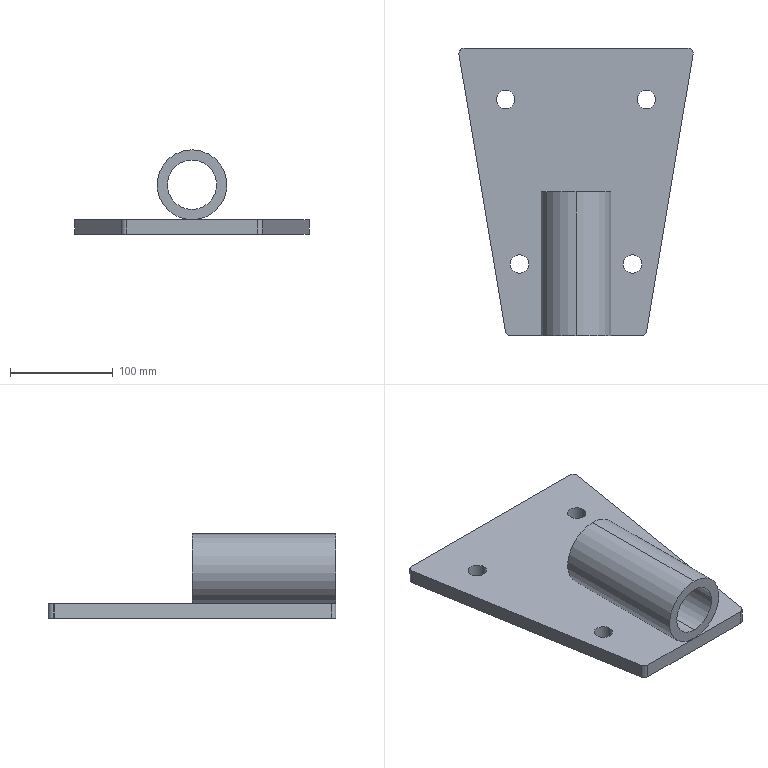Part | SolidWorks | features Extrusion 1, Fillet 1, HoleWzd 1, ICE 1 | 2 solids | 25 faces | box 227.837 x 280 x 82 mm | volume 957079 mm3 | cylinder 17 | plane 8 | commonest cylinder face diameters 18 x8 10 x5 48 x2 68 x2
STEP:
#1=CARTESIAN_POINT('',(0.,-2195.,72.));
#2=VERTEX_POINT('',#1);
#3=CARTESIAN_POINT('',(0.,-2195.,24.));
#4=VERTEX_POINT('',#3);
#5=CARTESIAN_POINT('',(0.,-2195.,48.));
#6=DIRECTION('',(0.,-1.,0.));
#7=DIRECTION('',(0.,0.,-1.));
#8=AXIS2_PLACEMENT_3D('',#5,#6,#7);
#9=CIRCLE('',#8,24.);
#10=EDGE_CURVE('',#2,#4,#9,.T.);
#11=ORIENTED_EDGE('',*,*,#10,.F.);
#12=CARTESIAN_POINT('',(0.,-2335.,72.));
#13=VERTEX_POINT('',#12);
#14=CARTESIAN_POINT('',(0.,-2195.,72.));
#15=DIRECTION('',(0.,-1.,0.));
#16=VECTOR('',#15,1000.);
#17=LINE('',#14,#16);
#18=EDGE_CURVE('',#2,#13,#17,.T.);
#19=ORIENTED_EDGE('',*,*,#18,.T.);
#20=CARTESIAN_POINT('',(0.,-2335.,24.));
#21=VERTEX_POINT('',#20);
#22=CARTESIAN_POINT('',(0.,-2335.,48.));
#23=DIRECTION('',(0.,-1.,0.));
#24=DIRECTION('',(0.,0.,-1.));
#25=AXIS2_PLACEMENT_3D('',#22,#23,#24);
#26=CIRCLE('',#25,24.);
#27=EDGE_CURVE('',#13,#21,#26,.T.);
#28=ORIENTED_EDGE('',*,*,#27,.T.);
#29=CARTESIAN_POINT('',(0.,-2195.,24.));
#30=DIRECTION('',(0.,-1.,0.));
#31=VECTOR('',#30,1000.);
#32=LINE('',#29,#31);
#33=EDGE_CURVE('',#4,#21,#32,.T.);
#34=ORIENTED_EDGE('',*,*,#33,.F.);
#35=EDGE_LOOP('',(#11,#19,#28,#34));
#36=FACE_OUTER_BOUND('',#35,.T.);
#37=CARTESIAN_POINT('',(0.,-2195.,48.));
#38=DIRECTION('',(0.,-1.,0.));
#39=DIRECTION('',(0.,0.,-1.));
#40=AXIS2_PLACEMENT_3D('',#37,#38,#39);
#41=CYLINDRICAL_SURFACE('',#40,24.);
#42=ADVANCED_FACE('',(#36),#41,.F.);
#43=CARTESIAN_POINT('',(0.,-2195.,14.));
#44=VERTEX_POINT('',#43);
#45=CARTESIAN_POINT('',(0.,-2195.,82.));
#46=VERTEX_POINT('',#45);
#47=CARTESIAN_POINT('',(0.,-2195.,48.));
#48=DIRECTION('',(0.,-1.,0.));
#49=DIRECTION('',(0.,0.,-1.));
#50=AXIS2_PLACEMENT_3D('',#47,#48,#49);
#51=CIRCLE('',#50,34.);
#52=EDGE_CURVE('',#44,#46,#51,.T.);
#53=ORIENTED_EDGE('',*,*,#52,.T.);
#54=CARTESIAN_POINT('',(0.,-2335.,82.));
#55=VERTEX_POINT('',#54);
#56=CARTESIAN_POINT('',(0.,-2195.,82.));
#57=DIRECTION('',(0.,-1.,0.));
#58=VECTOR('',#57,1000.);
#59=LINE('',#56,#58);
#60=EDGE_CURVE('',#46,#55,#59,.T.);
#61=ORIENTED_EDGE('',*,*,#60,.T.);
#62=CARTESIAN_POINT('',(0.,-2335.,14.));
#63=VERTEX_POINT('',#62);
#64=CARTESIAN_POINT('',(0.,-2335.,48.));
#65=DIRECTION('',(0.,-1.,0.));
#66=DIRECTION('',(0.,0.,-1.));
#67=AXIS2_PLACEMENT_3D('',#64,#65,#66);
#68=CIRCLE('',#67,34.);
#69=EDGE_CURVE('',#63,#55,#68,.T.);
#70=ORIENTED_EDGE('',*,*,#69,.F.);
#71=CARTESIAN_POINT('',(0.,-2195.,14.));
#72=DIRECTION('',(0.,-1.,0.));
#73=VECTOR('',#72,1000.);
#74=LINE('',#71,#73);
#75=EDGE_CURVE('',#44,#63,#74,.T.);
#76=ORIENTED_EDGE('',*,*,#75,.F.);
#77=EDGE_LOOP('',(#53,#61,#70,#76));
#78=FACE_OUTER_BOUND('',#77,.T.);
#79=CARTESIAN_POINT('',(0.,-2195.,48.));
#80=DIRECTION('',(0.,-1.,0.));
#81=DIRECTION('',(0.,0.,-1.));
#82=AXIS2_PLACEMENT_3D('',#79,#80,#81);
#83=CYLINDRICAL_SURFACE('',#82,34.);
#84=ADVANCED_FACE('',(#78),#83,.T.);
#85=ORIENTED_EDGE('',*,*,#60,.F.);
#86=CARTESIAN_POINT('',(0.,-2195.,48.));
#87=DIRECTION('',(0.,-1.,0.));
#88=DIRECTION('',(0.,0.,-1.));
#89=AXIS2_PLACEMENT_3D('',#86,#87,#88);
#90=CIRCLE('',#89,34.);
#91=EDGE_CURVE('',#46,#44,#90,.T.);
#92=ORIENTED_EDGE('',*,*,#91,.T.);
#93=ORIENTED_EDGE('',*,*,#75,.T.);
#94=CARTESIAN_POINT('',(0.,-2335.,48.));
#95=DIRECTION('',(0.,-1.,0.));
#96=DIRECTION('',(0.,0.,-1.));
#97=AXIS2_PLACEMENT_3D('',#94,#95,#96);
#98=CIRCLE('',#97,34.);
#99=EDGE_CURVE('',#55,#63,#98,.T.);
#100=ORIENTED_EDGE('',*,*,#99,.F.);
#101=EDGE_LOOP('',(#85,#92,#93,#100));
#102=FACE_OUTER_BOUND('',#101,.T.);
#103=CARTESIAN_POINT('',(0.,-2195.,48.));
#104=DIRECTION('',(0.,-1.,0.));
#105=DIRECTION('',(0.,0.,-1.));
#106=AXIS2_PLACEMENT_3D('',#103,#104,#105);
#107=CYLINDRICAL_SURFACE('',#106,34.);
#108=ADVANCED_FACE('',(#102),#107,.T.);
#109=CARTESIAN_POINT('',(0.,-2195.,48.));
#110=DIRECTION('',(0.,-1.,0.));
#111=DIRECTION('',(0.,0.,-1.));
#112=AXIS2_PLACEMENT_3D('',#109,#110,#111);
#113=CIRCLE('',#112,24.);
#114=EDGE_CURVE('',#4,#2,#113,.T.);
#115=ORIENTED_EDGE('',*,*,#114,.T.);
#116=ORIENTED_EDGE('',*,*,#10,.T.);
#117=EDGE_LOOP('',(#115,#116));
#118=FACE_BOUND('',#117,.T.);
#119=ORIENTED_EDGE('',*,*,#52,.F.);
#120=ORIENTED_EDGE('',*,*,#91,.F.);
#121=EDGE_LOOP('',(#119,#120));
#122=FACE_OUTER_BOUND('',#121,.T.);
#123=CARTESIAN_POINT('',(0.,-2195.,48.));
#124=DIRECTION('',(0.,-1.,0.));
#125=DIRECTION('',(0.,0.,-1.));
#126=AXIS2_PLACEMENT_3D('',#123,#124,#125);
#127=PLANE('',#126);
#128=ADVANCED_FACE('',(#118,#122),#127,.F.);
#129=CARTESIAN_POINT('',(0.,-2335.,48.));
#130=DIRECTION('',(0.,-1.,0.));
#131=DIRECTION('',(0.,0.,-1.));
#132=AXIS2_PLACEMENT_3D('',#129,#130,#131);
#133=CIRCLE('',#132,24.);
#134=EDGE_CURVE('',#21,#13,#133,.T.);
#135=ORIENTED_EDGE('',*,*,#134,.F.);
#136=ORIENTED_EDGE('',*,*,#27,.F.);
#137=EDGE_LOOP('',(#135,#136));
#138=FACE_BOUND('',#137,.T.);
#139=ORIENTED_EDGE('',*,*,#69,.T.);
#140=ORIENTED_EDGE('',*,*,#99,.T.);
#141=EDGE_LOOP('',(#139,#140));
#142=FACE_OUTER_BOUND('',#141,.T.);
#143=CARTESIAN_POINT('',(0.,-2335.,48.));
#144=DIRECTION('',(0.,-1.,0.));
#145=DIRECTION('',(0.,0.,-1.));
#146=AXIS2_PLACEMENT_3D('',#143,#144,#145);
#147=PLANE('',#146);
#148=ADVANCED_FACE('',(#138,#142),#147,.T.);
#149=ORIENTED_EDGE('',*,*,#18,.F.);
#150=ORIENTED_EDGE('',*,*,#114,.F.);
#151=ORIENTED_EDGE('',*,*,#33,.T.);
#152=ORIENTED_EDGE('',*,*,#134,.T.);
#153=EDGE_LOOP('',(#149,#150,#151,#152));
#154=FACE_OUTER_BOUND('',#153,.T.);
#155=CARTESIAN_POINT('',(0.,-2195.,48.));
#156=DIRECTION('',(0.,-1.,0.));
#157=DIRECTION('',(0.,0.,-1.));
#158=AXIS2_PLACEMENT_3D('',#155,#156,#157);
#159=CYLINDRICAL_SURFACE('',#158,24.);
#160=ADVANCED_FACE('',(#154),#159,.F.);
#161=CLOSED_SHELL('',(#42,#84,#108,#128,#148,#160));
#162=MANIFOLD_SOLID_BREP('',#161);
#163=CARTESIAN_POINT('',(59.437,-2105.,14.));
#164=VERTEX_POINT('',#163);
#165=CARTESIAN_POINT('',(77.437,-2105.,14.));
#166=VERTEX_POINT('',#165);
#167=CARTESIAN_POINT('',(68.437,-2105.,14.));
#168=DIRECTION('',(0.,0.,1.));
#169=DIRECTION('',(1.,0.,0.));
#170=AXIS2_PLACEMENT_3D('',#167,#168,#169);
#171=CIRCLE('',#170,9.);
#172=EDGE_CURVE('',#164,#166,#171,.T.);
#173=ORIENTED_EDGE('',*,*,#172,.T.);
#174=CARTESIAN_POINT('',(77.437,-2105.,0.));
#175=VERTEX_POINT('',#174);
#176=CARTESIAN_POINT('',(77.437,-2105.,0.));
#177=DIRECTION('',(0.,0.,-1.));
#178=VECTOR('',#177,1000.);
#179=LINE('',#176,#178);
#180=EDGE_CURVE('',#166,#175,#179,.T.);
#181=ORIENTED_EDGE('',*,*,#180,.T.);
#182=CARTESIAN_POINT('',(59.437,-2105.,0.));
#183=VERTEX_POINT('',#182);
#184=CARTESIAN_POINT('',(68.437,-2105.,0.));
#185=DIRECTION('',(0.,0.,-1.));
#186=DIRECTION('',(-1.,0.,0.));
#187=AXIS2_PLACEMENT_3D('',#184,#185,#186);
#188=CIRCLE('',#187,9.);
#189=EDGE_CURVE('',#175,#183,#188,.T.);
#190=ORIENTED_EDGE('',*,*,#189,.T.);
#191=CARTESIAN_POINT('',(59.437,-2105.,0.));
#192=DIRECTION('',(0.,0.,-1.));
#193=VECTOR('',#192,1000.);
#194=LINE('',#191,#193);
#195=EDGE_CURVE('',#164,#183,#194,.T.);
#196=ORIENTED_EDGE('',*,*,#195,.F.);
#197=EDGE_LOOP('',(#173,#181,#190,#196));
#198=FACE_OUTER_BOUND('',#197,.T.);
#199=CARTESIAN_POINT('',(68.437,-2105.,0.));
#200=DIRECTION('',(0.,0.,-1.));
#201=DIRECTION('',(-1.,0.,0.));
#202=AXIS2_PLACEMENT_3D('',#199,#200,#201);
#203=CYLINDRICAL_SURFACE('',#202,9.);
#204=ADVANCED_FACE('',(#198),#203,.F.);
#205=CARTESIAN_POINT('',(46.,-2265.,14.));
#206=VERTEX_POINT('',#205);
#207=CARTESIAN_POINT('',(64.,-2265.,14.));
#208=VERTEX_POINT('',#207);
#209=CARTESIAN_POINT('',(55.,-2265.,14.));
#210=DIRECTION('',(0.,0.,1.));
#211=DIRECTION('',(1.,0.,0.));
#212=AXIS2_PLACEMENT_3D('',#209,#210,#211);
#213=CIRCLE('',#212,9.);
#214=EDGE_CURVE('',#206,#208,#213,.T.);
#215=ORIENTED_EDGE('',*,*,#214,.T.);
#216=CARTESIAN_POINT('',(64.,-2265.,0.));
#217=VERTEX_POINT('',#216);
#218=CARTESIAN_POINT('',(64.,-2265.,0.));
#219=DIRECTION('',(0.,0.,-1.));
#220=VECTOR('',#219,1000.);
#221=LINE('',#218,#220);
#222=EDGE_CURVE('',#208,#217,#221,.T.);
#223=ORIENTED_EDGE('',*,*,#222,.T.);
#224=CARTESIAN_POINT('',(46.,-2265.,0.));
#225=VERTEX_POINT('',#224);
#226=CARTESIAN_POINT('',(55.,-2265.,0.));
#227=DIRECTION('',(0.,0.,-1.));
#228=DIRECTION('',(-1.,0.,0.));
#229=AXIS2_PLACEMENT_3D('',#226,#227,#228);
#230=CIRCLE('',#229,9.);
#231=EDGE_CURVE('',#217,#225,#230,.T.);
#232=ORIENTED_EDGE('',*,*,#231,.T.);
#233=CARTESIAN_POINT('',(46.,-2265.,0.));
#234=DIRECTION('',(0.,0.,-1.));
#235=VECTOR('',#234,1000.);
#236=LINE('',#233,#235);
#237=EDGE_CURVE('',#206,#225,#236,.T.);
#238=ORIENTED_EDGE('',*,*,#237,.F.);
#239=EDGE_LOOP('',(#215,#223,#232,#238));
#240=FACE_OUTER_BOUND('',#239,.T.);
#241=CARTESIAN_POINT('',(55.,-2265.,0.));
#242=DIRECTION('',(0.,0.,-1.));
#243=DIRECTION('',(-1.,0.,0.));
#244=AXIS2_PLACEMENT_3D('',#241,#242,#243);
#245=CYLINDRICAL_SURFACE('',#244,9.);
#246=ADVANCED_FACE('',(#240),#245,.F.);
#247=CARTESIAN_POINT('',(-64.,-2265.,14.));
#248=VERTEX_POINT('',#247);
#249=CARTESIAN_POINT('',(-46.,-2265.,14.));
#250=VERTEX_POINT('',#249);
#251=CARTESIAN_POINT('',(-55.,-2265.,14.));
#252=DIRECTION('',(0.,0.,1.));
#253=DIRECTION('',(1.,0.,0.));
#254=AXIS2_PLACEMENT_3D('',#251,#252,#253);
#255=CIRCLE('',#254,9.);
#256=EDGE_CURVE('',#248,#250,#255,.T.);
#257=ORIENTED_EDGE('',*,*,#256,.T.);
#258=CARTESIAN_POINT('',(-46.,-2265.,0.));
#259=VERTEX_POINT('',#258);
#260=CARTESIAN_POINT('',(-46.,-2265.,0.));
#261=DIRECTION('',(0.,0.,-1.));
#262=VECTOR('',#261,1000.);
#263=LINE('',#260,#262);
#264=EDGE_CURVE('',#250,#259,#263,.T.);
#265=ORIENTED_EDGE('',*,*,#264,.T.);
#266=CARTESIAN_POINT('',(-64.,-2265.,0.));
#267=VERTEX_POINT('',#266);
#268=CARTESIAN_POINT('',(-55.,-2265.,0.));
#269=DIRECTION('',(0.,0.,-1.));
#270=DIRECTION('',(-1.,0.,0.));
#271=AXIS2_PLACEMENT_3D('',#268,#269,#270);
#272=CIRCLE('',#271,9.);
#273=EDGE_CURVE('',#259,#267,#272,.T.);
#274=ORIENTED_EDGE('',*,*,#273,.T.);
#275=CARTESIAN_POINT('',(-64.,-2265.,0.));
#276=DIRECTION('',(0.,0.,-1.));
#277=VECTOR('',#276,1000.);
#278=LINE('',#275,#277);
#279=EDGE_CURVE('',#248,#267,#278,.T.);
#280=ORIENTED_EDGE('',*,*,#279,.F.);
#281=EDGE_LOOP('',(#257,#265,#274,#280));
#282=FACE_OUTER_BOUND('',#281,.T.);
#283=CARTESIAN_POINT('',(-55.,-2265.,0.));
#284=DIRECTION('',(0.,0.,-1.));
#285=DIRECTION('',(-1.,0.,0.));
#286=AXIS2_PLACEMENT_3D('',#283,#284,#285);
#287=CYLINDRICAL_SURFACE('',#286,9.);
#288=ADVANCED_FACE('',(#282),#287,.F.);
#289=CARTESIAN_POINT('',(-77.437,-2105.,14.));
#290=VERTEX_POINT('',#289);
#291=CARTESIAN_POINT('',(-59.437,-2105.,14.));
#292=VERTEX_POINT('',#291);
#293=CARTESIAN_POINT('',(-68.437,-2105.,14.));
#294=DIRECTION('',(0.,0.,1.));
#295=DIRECTION('',(1.,0.,0.));
#296=AXIS2_PLACEMENT_3D('',#293,#294,#295);
#297=CIRCLE('',#296,9.);
#298=EDGE_CURVE('',#290,#292,#297,.T.);
#299=ORIENTED_EDGE('',*,*,#298,.T.);
#300=CARTESIAN_POINT('',(-59.437,-2105.,0.));
#301=VERTEX_POINT('',#300);
#302=CARTESIAN_POINT('',(-59.437,-2105.,0.));
#303=DIRECTION('',(0.,0.,-1.));
#304=VECTOR('',#303,1000.);
#305=LINE('',#302,#304);
#306=EDGE_CURVE('',#292,#301,#305,.T.);
#307=ORIENTED_EDGE('',*,*,#306,.T.);
#308=CARTESIAN_POINT('',(-77.437,-2105.,0.));
#309=VERTEX_POINT('',#308);
#310=CARTESIAN_POINT('',(-68.437,-2105.,0.));
#311=DIRECTION('',(0.,0.,-1.));
#312=DIRECTION('',(-1.,0.,0.));
#313=AXIS2_PLACEMENT_3D('',#310,#311,#312);
#314=CIRCLE('',#313,9.);
#315=EDGE_CURVE('',#301,#309,#314,.T.);
#316=ORIENTED_EDGE('',*,*,#315,.T.);
#317=CARTESIAN_POINT('',(-77.437,-2105.,0.));
#318=DIRECTION('',(0.,0.,-1.));
#319=VECTOR('',#318,1000.);
#320=LINE('',#317,#319);
#321=EDGE_CURVE('',#290,#309,#320,.T.);
#322=ORIENTED_EDGE('',*,*,#321,.F.);
#323=EDGE_LOOP('',(#299,#307,#316,#322));
#324=FACE_OUTER_BOUND('',#323,.T.);
#325=CARTESIAN_POINT('',(-68.437,-2105.,0.));
#326=DIRECTION('',(0.,0.,-1.));
#327=DIRECTION('',(-1.,0.,0.));
#328=AXIS2_PLACEMENT_3D('',#325,#326,#327);
#329=CYLINDRICAL_SURFACE('',#328,9.);
#330=ADVANCED_FACE('',(#324),#329,.F.);
#331=CARTESIAN_POINT('',(-113.919,-2060.,14.));
#332=VERTEX_POINT('',#331);
#333=CARTESIAN_POINT('',(-113.85,-2060.825,14.));
#334=VERTEX_POINT('',#333);
#335=CARTESIAN_POINT('',(-108.919,-2060.,14.));
#336=DIRECTION('',(0.,0.,1.));
#337=DIRECTION('',(1.,0.,0.));
#338=AXIS2_PLACEMENT_3D('',#335,#336,#337);
#339=CIRCLE('',#338,5.);
#340=EDGE_CURVE('',#332,#334,#339,.T.);
#341=ORIENTED_EDGE('',*,*,#340,.F.);
#342=CARTESIAN_POINT('',(-113.919,-2060.,0.));
#343=VERTEX_POINT('',#342);
#344=CARTESIAN_POINT('',(-113.919,-2060.,14.));
#345=DIRECTION('',(0.,0.,-1.));
#346=VECTOR('',#345,1000.);
#347=LINE('',#344,#346);
#348=EDGE_CURVE('',#332,#343,#347,.T.);
#349=ORIENTED_EDGE('',*,*,#348,.T.);
#350=CARTESIAN_POINT('',(-113.85,-2060.825,0.));
#351=VERTEX_POINT('',#350);
#352=CARTESIAN_POINT('',(-108.919,-2060.,0.));
#353=DIRECTION('',(0.,0.,-1.));
#354=DIRECTION('',(1.,0.,0.));
#355=AXIS2_PLACEMENT_3D('',#352,#353,#354);
#356=CIRCLE('',#355,5.);
#357=EDGE_CURVE('',#351,#343,#356,.T.);
#358=ORIENTED_EDGE('',*,*,#357,.F.);
#359=CARTESIAN_POINT('',(-113.85,-2060.825,14.));
#360=DIRECTION('',(0.,0.,-1.));
#361=VECTOR('',#360,1000.);
#362=LINE('',#359,#361);
#363=EDGE_CURVE('',#334,#351,#362,.T.);
#364=ORIENTED_EDGE('',*,*,#363,.F.);
#365=EDGE_LOOP('',(#341,#349,#358,#364));
#366=FACE_OUTER_BOUND('',#365,.T.);
#367=CARTESIAN_POINT('',(-108.919,-2060.,14.));
#368=DIRECTION('',(0.,0.,-1.));
#369=DIRECTION('',(-1.,0.,0.));
#370=AXIS2_PLACEMENT_3D('',#367,#368,#369);
#371=CYLINDRICAL_SURFACE('',#370,5.);
#372=ADVANCED_FACE('',(#366),#371,.T.);
#373=CARTESIAN_POINT('',(-68.668,-2330.825,14.));
#374=VERTEX_POINT('',#373);
#375=CARTESIAN_POINT('',(-114.825,-2055.,14.));
#376=DIRECTION('',(0.165,-0.9863,0.));
#377=VECTOR('',#376,1000.);
#378=LINE('',#375,#377);
#379=EDGE_CURVE('',#334,#374,#378,.T.);
#380=ORIENTED_EDGE('',*,*,#379,.F.);
#381=ORIENTED_EDGE('',*,*,#363,.T.);
#382=CARTESIAN_POINT('',(-68.668,-2330.825,0.));
#383=VERTEX_POINT('',#382);
#384=CARTESIAN_POINT('',(-114.825,-2055.,0.));
#385=DIRECTION('',(0.165,-0.9863,0.));
#386=VECTOR('',#385,1000.);
#387=LINE('',#384,#386);
#388=EDGE_CURVE('',#351,#383,#387,.T.);
#389=ORIENTED_EDGE('',*,*,#388,.T.);
#390=CARTESIAN_POINT('',(-68.668,-2330.825,14.));
#391=DIRECTION('',(0.,0.,1.));
#392=VECTOR('',#391,1000.);
#393=LINE('',#390,#392);
#394=EDGE_CURVE('',#383,#374,#393,.T.);
#395=ORIENTED_EDGE('',*,*,#394,.T.);
#396=EDGE_LOOP('',(#380,#381,#389,#395));
#397=FACE_OUTER_BOUND('',#396,.T.);
#398=CARTESIAN_POINT('',(-114.825,-2055.,14.));
#399=DIRECTION('',(0.9863,0.165,0.));
#400=DIRECTION('',(-0.165,0.9863,0.));
#401=AXIS2_PLACEMENT_3D('',#398,#399,#400);
#402=PLANE('',#401);
#403=ADVANCED_FACE('',(#397),#402,.F.);
#404=CARTESIAN_POINT('',(-63.736,-2335.,14.));
#405=VERTEX_POINT('',#404);
#406=CARTESIAN_POINT('',(63.736,-2335.,14.));
#407=VERTEX_POINT('',#406);
#408=CARTESIAN_POINT('',(-67.969,-2335.,14.));
#409=DIRECTION('',(1.,0.,0.));
#410=VECTOR('',#409,1000.);
#411=LINE('',#408,#410);
#412=EDGE_CURVE('',#405,#407,#411,.T.);
#413=ORIENTED_EDGE('',*,*,#412,.F.);
#414=CARTESIAN_POINT('',(-63.736,-2335.,0.));
#415=VERTEX_POINT('',#414);
#416=CARTESIAN_POINT('',(-63.736,-2335.,14.));
#417=DIRECTION('',(0.,0.,-1.));
#418=VECTOR('',#417,1000.);
#419=LINE('',#416,#418);
#420=EDGE_CURVE('',#405,#415,#419,.T.);
#421=ORIENTED_EDGE('',*,*,#420,.T.);
#422=CARTESIAN_POINT('',(63.736,-2335.,0.));
#423=VERTEX_POINT('',#422);
#424=CARTESIAN_POINT('',(-67.969,-2335.,0.));
#425=DIRECTION('',(1.,0.,0.));
#426=VECTOR('',#425,1000.);
#427=LINE('',#424,#426);
#428=EDGE_CURVE('',#415,#423,#427,.T.);
#429=ORIENTED_EDGE('',*,*,#428,.T.);
#430=CARTESIAN_POINT('',(63.736,-2335.,14.));
#431=DIRECTION('',(0.,0.,1.));
#432=VECTOR('',#431,1000.);
#433=LINE('',#430,#432);
#434=EDGE_CURVE('',#423,#407,#433,.T.);
#435=ORIENTED_EDGE('',*,*,#434,.T.);
#436=EDGE_LOOP('',(#413,#421,#429,#435));
#437=FACE_OUTER_BOUND('',#436,.T.);
#438=CARTESIAN_POINT('',(-67.969,-2335.,14.));
#439=DIRECTION('',(0.,1.,0.));
#440=DIRECTION('',(0.,0.,1.));
#441=AXIS2_PLACEMENT_3D('',#438,#439,#440);
#442=PLANE('',#441);
#443=ADVANCED_FACE('',(#437),#442,.F.);
#444=CARTESIAN_POINT('',(68.668,-2330.825,0.));
#445=VERTEX_POINT('',#444);
#446=CARTESIAN_POINT('',(113.85,-2060.825,0.));
#447=VERTEX_POINT('',#446);
#448=CARTESIAN_POINT('',(67.969,-2335.,0.));
#449=DIRECTION('',(0.165,0.9863,0.));
#450=VECTOR('',#449,1000.);
#451=LINE('',#448,#450);
#452=EDGE_CURVE('',#445,#447,#451,.T.);
#453=ORIENTED_EDGE('',*,*,#452,.T.);
#454=CARTESIAN_POINT('',(113.85,-2060.825,14.));
#455=VERTEX_POINT('',#454);
#456=CARTESIAN_POINT('',(113.85,-2060.825,14.));
#457=DIRECTION('',(0.,0.,1.));
#458=VECTOR('',#457,1000.);
#459=LINE('',#456,#458);
#460=EDGE_CURVE('',#447,#455,#459,.T.);
#461=ORIENTED_EDGE('',*,*,#460,.T.);
#462=CARTESIAN_POINT('',(68.668,-2330.825,14.));
#463=VERTEX_POINT('',#462);
#464=CARTESIAN_POINT('',(67.969,-2335.,14.));
#465=DIRECTION('',(0.165,0.9863,0.));
#466=VECTOR('',#465,1000.);
#467=LINE('',#464,#466);
#468=EDGE_CURVE('',#463,#455,#467,.T.);
#469=ORIENTED_EDGE('',*,*,#468,.F.);
#470=CARTESIAN_POINT('',(68.668,-2330.825,14.));
#471=DIRECTION('',(0.,0.,-1.));
#472=VECTOR('',#471,1000.);
#473=LINE('',#470,#472);
#474=EDGE_CURVE('',#463,#445,#473,.T.);
#475=ORIENTED_EDGE('',*,*,#474,.T.);
#476=EDGE_LOOP('',(#453,#461,#469,#475));
#477=FACE_OUTER_BOUND('',#476,.T.);
#478=CARTESIAN_POINT('',(67.969,-2335.,14.));
#479=DIRECTION('',(-0.9863,0.165,0.));
#480=DIRECTION('',(-0.165,-0.9863,0.));
#481=AXIS2_PLACEMENT_3D('',#478,#479,#480);
#482=PLANE('',#481);
#483=ADVANCED_FACE('',(#477),#482,.F.);
#484=CARTESIAN_POINT('',(108.919,-2055.,0.));
#485=VERTEX_POINT('',#484);
#486=CARTESIAN_POINT('',(-108.919,-2055.,0.));
#487=VERTEX_POINT('',#486);
#488=CARTESIAN_POINT('',(114.825,-2055.,0.));
#489=DIRECTION('',(-1.,0.,0.));
#490=VECTOR('',#489,1000.);
#491=LINE('',#488,#490);
#492=EDGE_CURVE('',#485,#487,#491,.T.);
#493=ORIENTED_EDGE('',*,*,#492,.T.);
#494=CARTESIAN_POINT('',(-108.919,-2055.,14.));
#495=VERTEX_POINT('',#494);
#496=CARTESIAN_POINT('',(-108.919,-2055.,14.));
#497=DIRECTION('',(0.,0.,1.));
#498=VECTOR('',#497,1000.);
#499=LINE('',#496,#498);
#500=EDGE_CURVE('',#487,#495,#499,.T.);
#501=ORIENTED_EDGE('',*,*,#500,.T.);
#502=CARTESIAN_POINT('',(108.919,-2055.,14.));
#503=VERTEX_POINT('',#502);
#504=CARTESIAN_POINT('',(114.825,-2055.,14.));
#505=DIRECTION('',(-1.,0.,0.));
#506=VECTOR('',#505,1000.);
#507=LINE('',#504,#506);
#508=EDGE_CURVE('',#503,#495,#507,.T.);
#509=ORIENTED_EDGE('',*,*,#508,.F.);
#510=CARTESIAN_POINT('',(108.919,-2055.,14.));
#511=DIRECTION('',(0.,0.,-1.));
#512=VECTOR('',#511,1000.);
#513=LINE('',#510,#512);
#514=EDGE_CURVE('',#503,#485,#513,.T.);
#515=ORIENTED_EDGE('',*,*,#514,.T.);
#516=EDGE_LOOP('',(#493,#501,#509,#515));
#517=FACE_OUTER_BOUND('',#516,.T.);
#518=CARTESIAN_POINT('',(114.825,-2055.,14.));
#519=DIRECTION('',(0.,-1.,0.));
#520=DIRECTION('',(0.,0.,-1.));
#521=AXIS2_PLACEMENT_3D('',#518,#519,#520);
#522=PLANE('',#521);
#523=ADVANCED_FACE('',(#517),#522,.F.);
#524=ORIENTED_EDGE('',*,*,#172,.F.);
#525=CARTESIAN_POINT('',(68.437,-2105.,14.));
#526=DIRECTION('',(0.,0.,1.));
#527=DIRECTION('',(1.,0.,0.));
#528=AXIS2_PLACEMENT_3D('',#525,#526,#527);
#529=CIRCLE('',#528,9.);
#530=EDGE_CURVE('',#166,#164,#529,.T.);
#531=ORIENTED_EDGE('',*,*,#530,.F.);
#532=EDGE_LOOP('',(#524,#531));
#533=FACE_BOUND('',#532,.T.);
#534=ORIENTED_EDGE('',*,*,#214,.F.);
#535=CARTESIAN_POINT('',(55.,-2265.,14.));
#536=DIRECTION('',(0.,0.,1.));
#537=DIRECTION('',(1.,0.,0.));
#538=AXIS2_PLACEMENT_3D('',#535,#536,#537);
#539=CIRCLE('',#538,9.);
#540=EDGE_CURVE('',#208,#206,#539,.T.);
#541=ORIENTED_EDGE('',*,*,#540,.F.);
#542=EDGE_LOOP('',(#534,#541));
#543=FACE_BOUND('',#542,.T.);
#544=ORIENTED_EDGE('',*,*,#256,.F.);
#545=CARTESIAN_POINT('',(-55.,-2265.,14.));
#546=DIRECTION('',(0.,0.,1.));
#547=DIRECTION('',(1.,0.,0.));
#548=AXIS2_PLACEMENT_3D('',#545,#546,#547);
#549=CIRCLE('',#548,9.);
#550=EDGE_CURVE('',#250,#248,#549,.T.);
#551=ORIENTED_EDGE('',*,*,#550,.F.);
#552=EDGE_LOOP('',(#544,#551));
#553=FACE_BOUND('',#552,.T.);
#554=ORIENTED_EDGE('',*,*,#298,.F.);
#555=CARTESIAN_POINT('',(-68.437,-2105.,14.));
#556=DIRECTION('',(0.,0.,1.));
#557=DIRECTION('',(1.,0.,0.));
#558=AXIS2_PLACEMENT_3D('',#555,#556,#557);
#559=CIRCLE('',#558,9.);
#560=EDGE_CURVE('',#292,#290,#559,.T.);
#561=ORIENTED_EDGE('',*,*,#560,.F.);
#562=EDGE_LOOP('',(#554,#561));
#563=FACE_BOUND('',#562,.T.);
#564=ORIENTED_EDGE('',*,*,#508,.T.);
#565=CARTESIAN_POINT('',(-108.919,-2060.,14.));
#566=DIRECTION('',(0.,0.,1.));
#567=DIRECTION('',(1.,0.,0.));
#568=AXIS2_PLACEMENT_3D('',#565,#566,#567);
#569=CIRCLE('',#568,5.);
#570=EDGE_CURVE('',#495,#332,#569,.T.);
#571=ORIENTED_EDGE('',*,*,#570,.T.);
#572=ORIENTED_EDGE('',*,*,#340,.T.);
#573=ORIENTED_EDGE('',*,*,#379,.T.);
#574=CARTESIAN_POINT('',(-63.736,-2330.,14.));
#575=DIRECTION('',(0.,0.,1.));
#576=DIRECTION('',(1.,0.,0.));
#577=AXIS2_PLACEMENT_3D('',#574,#575,#576);
#578=CIRCLE('',#577,5.);
#579=EDGE_CURVE('',#374,#405,#578,.T.);
#580=ORIENTED_EDGE('',*,*,#579,.T.);
#581=ORIENTED_EDGE('',*,*,#412,.T.);
#582=CARTESIAN_POINT('',(63.736,-2330.,14.));
#583=DIRECTION('',(0.,0.,1.));
#584=DIRECTION('',(1.,0.,0.));
#585=AXIS2_PLACEMENT_3D('',#582,#583,#584);
#586=CIRCLE('',#585,5.);
#587=EDGE_CURVE('',#407,#463,#586,.T.);
#588=ORIENTED_EDGE('',*,*,#587,.T.);
#589=ORIENTED_EDGE('',*,*,#468,.T.);
#590=CARTESIAN_POINT('',(108.919,-2060.,14.));
#591=DIRECTION('',(0.,0.,1.));
#592=DIRECTION('',(1.,0.,0.));
#593=AXIS2_PLACEMENT_3D('',#590,#591,#592);
#594=CIRCLE('',#593,5.);
#595=EDGE_CURVE('',#455,#503,#594,.T.);
#596=ORIENTED_EDGE('',*,*,#595,.T.);
#597=EDGE_LOOP('',(#564,#571,#572,#573,#580,#581,#588,#589,#596));
#598=FACE_OUTER_BOUND('',#597,.T.);
#599=CARTESIAN_POINT('',(0.,0.,14.));
#600=DIRECTION('',(0.,0.,1.));
#601=DIRECTION('',(1.,0.,0.));
#602=AXIS2_PLACEMENT_3D('',#599,#600,#601);
#603=PLANE('',#602);
#604=ADVANCED_FACE('',(#533,#543,#553,#563,#598),#603,.T.);
#605=CARTESIAN_POINT('',(68.437,-2105.,0.));
#606=DIRECTION('',(0.,0.,-1.));
#607=DIRECTION('',(-1.,0.,0.));
#608=AXIS2_PLACEMENT_3D('',#605,#606,#607);
#609=CIRCLE('',#608,9.);
#610=EDGE_CURVE('',#183,#175,#609,.T.);
#611=ORIENTED_EDGE('',*,*,#610,.F.);
#612=ORIENTED_EDGE('',*,*,#189,.F.);
#613=EDGE_LOOP('',(#611,#612));
#614=FACE_BOUND('',#613,.T.);
#615=CARTESIAN_POINT('',(55.,-2265.,0.));
#616=DIRECTION('',(0.,0.,-1.));
#617=DIRECTION('',(-1.,0.,0.));
#618=AXIS2_PLACEMENT_3D('',#615,#616,#617);
#619=CIRCLE('',#618,9.);
#620=EDGE_CURVE('',#225,#217,#619,.T.);
#621=ORIENTED_EDGE('',*,*,#620,.F.);
#622=ORIENTED_EDGE('',*,*,#231,.F.);
#623=EDGE_LOOP('',(#621,#622));
#624=FACE_BOUND('',#623,.T.);
#625=CARTESIAN_POINT('',(-55.,-2265.,0.));
#626=DIRECTION('',(0.,0.,-1.));
#627=DIRECTION('',(-1.,0.,0.));
#628=AXIS2_PLACEMENT_3D('',#625,#626,#627);
#629=CIRCLE('',#628,9.);
#630=EDGE_CURVE('',#267,#259,#629,.T.);
#631=ORIENTED_EDGE('',*,*,#630,.F.);
#632=ORIENTED_EDGE('',*,*,#273,.F.);
#633=EDGE_LOOP('',(#631,#632));
#634=FACE_BOUND('',#633,.T.);
#635=CARTESIAN_POINT('',(-68.437,-2105.,0.));
#636=DIRECTION('',(0.,0.,-1.));
#637=DIRECTION('',(-1.,0.,0.));
#638=AXIS2_PLACEMENT_3D('',#635,#636,#637);
#639=CIRCLE('',#638,9.);
#640=EDGE_CURVE('',#309,#301,#639,.T.);
#641=ORIENTED_EDGE('',*,*,#640,.F.);
#642=ORIENTED_EDGE('',*,*,#315,.F.);
#643=EDGE_LOOP('',(#641,#642));
#644=FACE_BOUND('',#643,.T.);
#645=ORIENTED_EDGE('',*,*,#388,.F.);
#646=ORIENTED_EDGE('',*,*,#357,.T.);
#647=CARTESIAN_POINT('',(-108.919,-2060.,0.));
#648=DIRECTION('',(0.,0.,-1.));
#649=DIRECTION('',(1.,0.,0.));
#650=AXIS2_PLACEMENT_3D('',#647,#648,#649);
#651=CIRCLE('',#650,5.);
#652=EDGE_CURVE('',#343,#487,#651,.T.);
#653=ORIENTED_EDGE('',*,*,#652,.T.);
#654=ORIENTED_EDGE('',*,*,#492,.F.);
#655=CARTESIAN_POINT('',(108.919,-2060.,0.));
#656=DIRECTION('',(0.,0.,-1.));
#657=DIRECTION('',(1.,0.,0.));
#658=AXIS2_PLACEMENT_3D('',#655,#656,#657);
#659=CIRCLE('',#658,5.);
#660=EDGE_CURVE('',#485,#447,#659,.T.);
#661=ORIENTED_EDGE('',*,*,#660,.T.);
#662=ORIENTED_EDGE('',*,*,#452,.F.);
#663=CARTESIAN_POINT('',(63.736,-2330.,0.));
#664=DIRECTION('',(0.,0.,-1.));
#665=DIRECTION('',(1.,0.,0.));
#666=AXIS2_PLACEMENT_3D('',#663,#664,#665);
#667=CIRCLE('',#666,5.);
#668=EDGE_CURVE('',#445,#423,#667,.T.);
#669=ORIENTED_EDGE('',*,*,#668,.T.);
#670=ORIENTED_EDGE('',*,*,#428,.F.);
#671=CARTESIAN_POINT('',(-63.736,-2330.,0.));
#672=DIRECTION('',(0.,0.,-1.));
#673=DIRECTION('',(1.,0.,0.));
#674=AXIS2_PLACEMENT_3D('',#671,#672,#673);
#675=CIRCLE('',#674,5.);
#676=EDGE_CURVE('',#415,#383,#675,.T.);
#677=ORIENTED_EDGE('',*,*,#676,.T.);
#678=EDGE_LOOP('',(#645,#646,#653,#654,#661,#662,#669,#670,#677));
#679=FACE_OUTER_BOUND('',#678,.T.);
#680=CARTESIAN_POINT('',(0.,0.,0.));
#681=DIRECTION('',(0.,0.,1.));
#682=DIRECTION('',(1.,0.,0.));
#683=AXIS2_PLACEMENT_3D('',#680,#681,#682);
#684=PLANE('',#683);
#685=ADVANCED_FACE('',(#614,#624,#634,#644,#679),#684,.F.);
#686=ORIENTED_EDGE('',*,*,#348,.F.);
#687=ORIENTED_EDGE('',*,*,#570,.F.);
#688=ORIENTED_EDGE('',*,*,#500,.F.);
#689=ORIENTED_EDGE('',*,*,#652,.F.);
#690=EDGE_LOOP('',(#686,#687,#688,#689));
#691=FACE_OUTER_BOUND('',#690,.T.);
#692=CARTESIAN_POINT('',(-108.919,-2060.,14.));
#693=DIRECTION('',(0.,0.,-1.));
#694=DIRECTION('',(-1.,0.,0.));
#695=AXIS2_PLACEMENT_3D('',#692,#693,#694);
#696=CYLINDRICAL_SURFACE('',#695,5.);
#697=ADVANCED_FACE('',(#691),#696,.T.);
#698=ORIENTED_EDGE('',*,*,#595,.F.);
#699=ORIENTED_EDGE('',*,*,#460,.F.);
#700=ORIENTED_EDGE('',*,*,#660,.F.);
#701=ORIENTED_EDGE('',*,*,#514,.F.);
#702=EDGE_LOOP('',(#698,#699,#700,#701));
#703=FACE_OUTER_BOUND('',#702,.T.);
#704=CARTESIAN_POINT('',(108.919,-2060.,14.));
#705=DIRECTION('',(0.,0.,-1.));
#706=DIRECTION('',(-1.,0.,0.));
#707=AXIS2_PLACEMENT_3D('',#704,#705,#706);
#708=CYLINDRICAL_SURFACE('',#707,5.);
#709=ADVANCED_FACE('',(#703),#708,.T.);
#710=ORIENTED_EDGE('',*,*,#579,.F.);
#711=ORIENTED_EDGE('',*,*,#394,.F.);
#712=ORIENTED_EDGE('',*,*,#676,.F.);
#713=ORIENTED_EDGE('',*,*,#420,.F.);
#714=EDGE_LOOP('',(#710,#711,#712,#713));
#715=FACE_OUTER_BOUND('',#714,.T.);
#716=CARTESIAN_POINT('',(-63.736,-2330.,14.));
#717=DIRECTION('',(0.,0.,-1.));
#718=DIRECTION('',(-1.,0.,0.));
#719=AXIS2_PLACEMENT_3D('',#716,#717,#718);
#720=CYLINDRICAL_SURFACE('',#719,5.);
#721=ADVANCED_FACE('',(#715),#720,.T.);
#722=ORIENTED_EDGE('',*,*,#587,.F.);
#723=ORIENTED_EDGE('',*,*,#434,.F.);
#724=ORIENTED_EDGE('',*,*,#668,.F.);
#725=ORIENTED_EDGE('',*,*,#474,.F.);
#726=EDGE_LOOP('',(#722,#723,#724,#725));
#727=FACE_OUTER_BOUND('',#726,.T.);
#728=CARTESIAN_POINT('',(63.736,-2330.,14.));
#729=DIRECTION('',(0.,0.,-1.));
#730=DIRECTION('',(-1.,0.,0.));
#731=AXIS2_PLACEMENT_3D('',#728,#729,#730);
#732=CYLINDRICAL_SURFACE('',#731,5.);
#733=ADVANCED_FACE('',(#727),#732,.T.);
#734=ORIENTED_EDGE('',*,*,#306,.F.);
#735=ORIENTED_EDGE('',*,*,#560,.T.);
#736=ORIENTED_EDGE('',*,*,#321,.T.);
#737=ORIENTED_EDGE('',*,*,#640,.T.);
#738=EDGE_LOOP('',(#734,#735,#736,#737));
#739=FACE_OUTER_BOUND('',#738,.T.);
#740=CARTESIAN_POINT('',(-68.437,-2105.,0.));
#741=DIRECTION('',(0.,0.,-1.));
#742=DIRECTION('',(-1.,0.,0.));
#743=AXIS2_PLACEMENT_3D('',#740,#741,#742);
#744=CYLINDRICAL_SURFACE('',#743,9.);
#745=ADVANCED_FACE('',(#739),#744,.F.);
#746=ORIENTED_EDGE('',*,*,#264,.F.);
#747=ORIENTED_EDGE('',*,*,#550,.T.);
#748=ORIENTED_EDGE('',*,*,#279,.T.);
#749=ORIENTED_EDGE('',*,*,#630,.T.);
#750=EDGE_LOOP('',(#746,#747,#748,#749));
#751=FACE_OUTER_BOUND('',#750,.T.);
#752=CARTESIAN_POINT('',(-55.,-2265.,0.));
#753=DIRECTION('',(0.,0.,-1.));
#754=DIRECTION('',(-1.,0.,0.));
#755=AXIS2_PLACEMENT_3D('',#752,#753,#754);
#756=CYLINDRICAL_SURFACE('',#755,9.);
#757=ADVANCED_FACE('',(#751),#756,.F.);
#758=ORIENTED_EDGE('',*,*,#222,.F.);
#759=ORIENTED_EDGE('',*,*,#540,.T.);
#760=ORIENTED_EDGE('',*,*,#237,.T.);
#761=ORIENTED_EDGE('',*,*,#620,.T.);
#762=EDGE_LOOP('',(#758,#759,#760,#761));
#763=FACE_OUTER_BOUND('',#762,.T.);
#764=CARTESIAN_POINT('',(55.,-2265.,0.));
#765=DIRECTION('',(0.,0.,-1.));
#766=DIRECTION('',(-1.,0.,0.));
#767=AXIS2_PLACEMENT_3D('',#764,#765,#766);
#768=CYLINDRICAL_SURFACE('',#767,9.);
#769=ADVANCED_FACE('',(#763),#768,.F.);
#770=ORIENTED_EDGE('',*,*,#180,.F.);
#771=ORIENTED_EDGE('',*,*,#530,.T.);
#772=ORIENTED_EDGE('',*,*,#195,.T.);
#773=ORIENTED_EDGE('',*,*,#610,.T.);
#774=EDGE_LOOP('',(#770,#771,#772,#773));
#775=FACE_OUTER_BOUND('',#774,.T.);
#776=CARTESIAN_POINT('',(68.437,-2105.,0.));
#777=DIRECTION('',(0.,0.,-1.));
#778=DIRECTION('',(-1.,0.,0.));
#779=AXIS2_PLACEMENT_3D('',#776,#777,#778);
#780=CYLINDRICAL_SURFACE('',#779,9.);
#781=ADVANCED_FACE('',(#775),#780,.F.);
#782=CLOSED_SHELL('',(#204,#246,#288,#330,#372,#403,#443,#483,#523,#604,#685,#697,#709,#721,#733,#745,#757,#769,#781));
#783=MANIFOLD_SOLID_BREP('',#782);
#784=CARTESIAN_POINT('',(0.,0.,0.));
#785=DIRECTION('',(0.,0.,1.));
#786=DIRECTION('',(1.,0.,0.));
#787=AXIS2_PLACEMENT_3D('',#784,#785,#786);
#788=(LENGTH_UNIT()NAMED_UNIT(*)SI_UNIT(.MILLI.,.METRE.));
#789=UNCERTAINTY_MEASURE_WITH_UNIT(LENGTH_MEASURE(0.00001),#788,'','');
#790=(NAMED_UNIT(*)PLANE_ANGLE_UNIT()SI_UNIT($,.RADIAN.));
#791=(NAMED_UNIT(*)SI_UNIT($,.STERADIAN.)SOLID_ANGLE_UNIT());
#792=(GEOMETRIC_REPRESENTATION_CONTEXT(3)GLOBAL_UNCERTAINTY_ASSIGNED_CONTEXT((#789))GLOBAL_UNIT_ASSIGNED_CONTEXT((#788,#790,#791))REPRESENTATION_CONTEXT('',''));
#793=ADVANCED_BREP_SHAPE_REPRESENTATION('',(#162,#783,#787),#792);